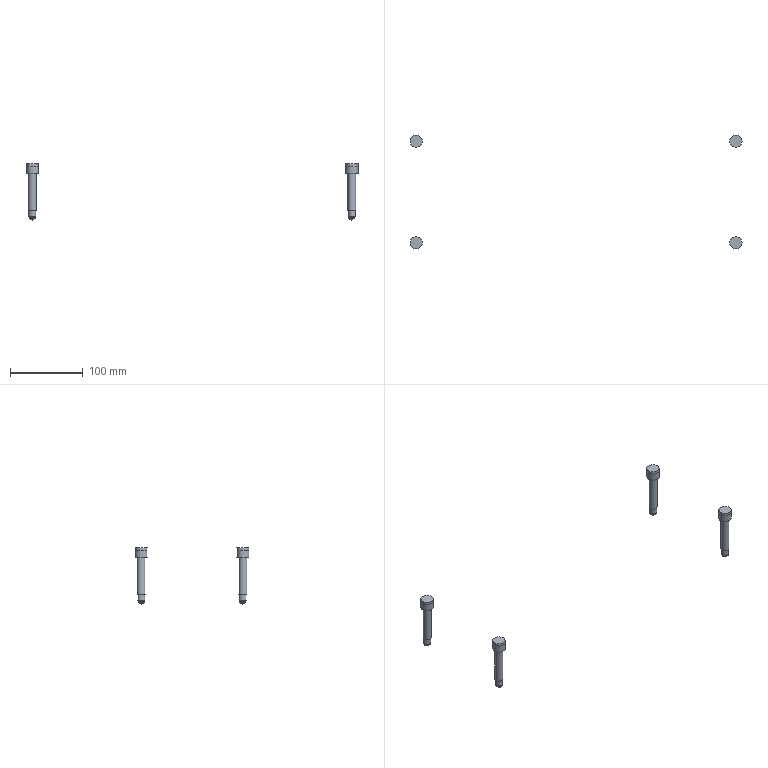Part | NX | features BREP 2 | 8 solids | 84 faces | box 457 x 157 x 78.231 mm | volume 60137 mm3 | plane 56 | cylinder 20 | cone 8 | commonest cylinder face diameters 8.5 x4 10 x4 11 x4 16 x4 17 x4